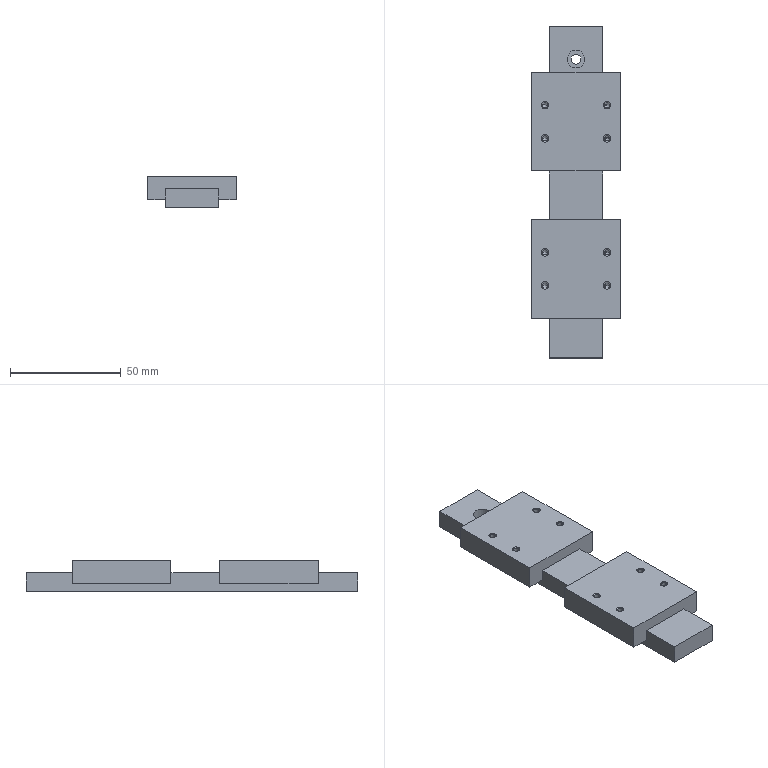Part | NX | 1 solid | 75 faces | box 40 x 150 x 14 mm | volume 56785 mm3 | cone 32 | plane 23 | cylinder 20 | commonest cylinder face diameters 2.5 x16 4.5 x2 8 x2